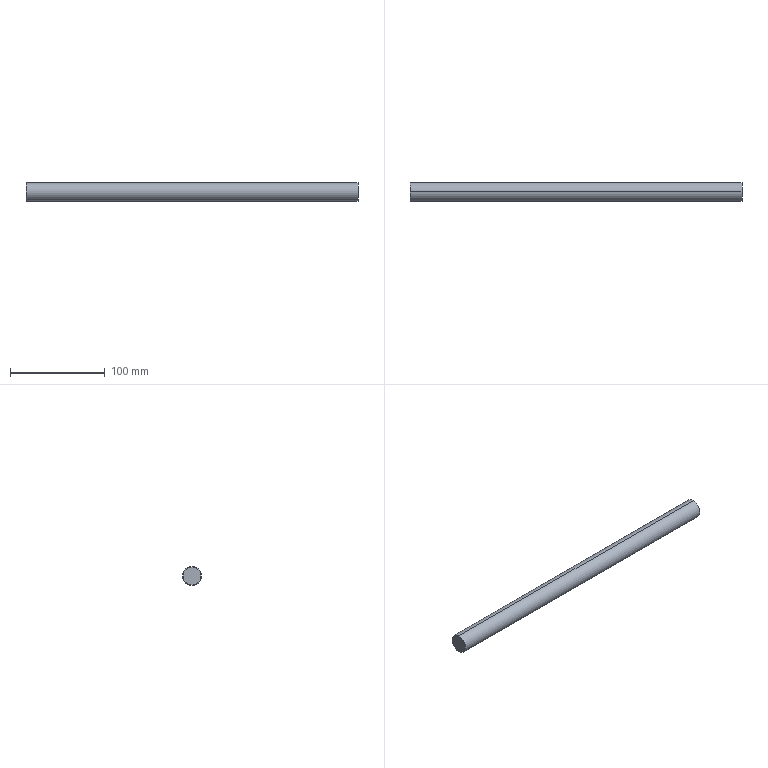Part | STEP file | Hold-down sync guide rod | 1 solid | 10 faces | box 350 x 20 x 20 mm | volume 109206 mm3 | cylinder 4 | cone 4 | plane 2 | commonest cylinder face diameters 6.8 x2 20 x2
STEP:
#1=CARTESIAN_POINT('',(0.,0.,0.));
#2=DIRECTION('',(0.,0.,1.));
#3=DIRECTION('',(1.,0.,0.));
#4=AXIS2_PLACEMENT_3D('',#1,#2,#3);
#5=CARTESIAN_POINT('',(330.25,18.056,30.521));
#6=VERTEX_POINT('',#5);
#7=CARTESIAN_POINT('',(350.,18.056,30.521));
#8=VERTEX_POINT('',#7);
#9=CARTESIAN_POINT('',(350.,18.056,30.521));
#10=DIRECTION('',(1.,0.,0.));
#11=VECTOR('',#10,1.);
#12=LINE('',#9,#11);
#13=CARTESIAN_POINT('',(350.,18.056,33.921));
#14=DIRECTION('',(1.,0.,0.));
#15=DIRECTION('',(0.,0.,-1.));
#16=AXIS2_PLACEMENT_3D('',#13,#14,#15);
#17=CYLINDRICAL_SURFACE('',#16,3.4);
#18=CARTESIAN_POINT('',(6.283,0.));
#19=DIRECTION('',(0.,1.));
#20=VECTOR('',#19,1.);
#21=LINE('',#18,#20);
#22=(GEOMETRIC_REPRESENTATION_CONTEXT(2)PARAMETRIC_REPRESENTATION_CONTEXT()REPRESENTATION_CONTEXT('',''));
#23=DEFINITIONAL_REPRESENTATION('',(#21),#22);
#24=PCURVE('',#17,#23);
#25=CARTESIAN_POINT('',(350.,18.056,33.921));
#26=DIRECTION('',(1.,0.,0.));
#27=DIRECTION('',(0.,0.,-1.));
#28=AXIS2_PLACEMENT_3D('',#25,#26,#27);
#29=CYLINDRICAL_SURFACE('',#28,3.4);
#30=CARTESIAN_POINT('',(0.,0.));
#31=DIRECTION('',(0.,1.));
#32=VECTOR('',#31,1.);
#33=LINE('',#30,#32);
#34=(GEOMETRIC_REPRESENTATION_CONTEXT(2)PARAMETRIC_REPRESENTATION_CONTEXT()REPRESENTATION_CONTEXT('',''));
#35=DEFINITIONAL_REPRESENTATION('',(#33),#34);
#36=PCURVE('',#29,#35);
#37=SURFACE_CURVE('',#12,(#24,#36),.PCURVE_S1.);
#38=EDGE_CURVE('',#6,#8,#37,.T.);
#39=ORIENTED_EDGE('',*,*,#38,.T.);
#40=CARTESIAN_POINT('',(350.,18.056,37.321));
#41=VERTEX_POINT('',#40);
#42=CARTESIAN_POINT('',(350.,18.056,33.921));
#43=DIRECTION('',(1.,0.,0.));
#44=DIRECTION('',(0.,0.,-1.));
#45=AXIS2_PLACEMENT_3D('',#42,#43,#44);
#46=CIRCLE('',#45,3.4);
#47=CARTESIAN_POINT('',(0.,0.));
#48=DIRECTION('',(1.,0.));
#49=VECTOR('',#48,1.);
#50=LINE('',#47,#49);
#51=(GEOMETRIC_REPRESENTATION_CONTEXT(2)PARAMETRIC_REPRESENTATION_CONTEXT()REPRESENTATION_CONTEXT('',''));
#52=DEFINITIONAL_REPRESENTATION('',(#50),#51);
#53=PCURVE('',#17,#52);
#54=CARTESIAN_POINT('',(350.,18.056,33.921));
#55=DIRECTION('',(1.,0.,0.));
#56=DIRECTION('',(0.,0.,-1.));
#57=AXIS2_PLACEMENT_3D('',#54,#55,#56);
#58=PLANE('',#57);
#59=CARTESIAN_POINT('',(0.,0.));
#60=DIRECTION('',(1.,0.));
#61=AXIS2_PLACEMENT_2D('',#59,#60);
#62=CIRCLE('',#61,3.4);
#63=(GEOMETRIC_REPRESENTATION_CONTEXT(2)PARAMETRIC_REPRESENTATION_CONTEXT()REPRESENTATION_CONTEXT('',''));
#64=DEFINITIONAL_REPRESENTATION('',(#62),#63);
#65=PCURVE('',#58,#64);
#66=SURFACE_CURVE('',#46,(#53,#65),.PCURVE_S1.);
#67=EDGE_CURVE('',#41,#8,#66,.T.);
#68=ORIENTED_EDGE('',*,*,#67,.F.);
#69=CARTESIAN_POINT('',(330.25,18.056,37.321));
#70=VERTEX_POINT('',#69);
#71=CARTESIAN_POINT('',(350.,18.056,37.321));
#72=DIRECTION('',(1.,0.,0.));
#73=VECTOR('',#72,1.);
#74=LINE('',#71,#73);
#75=CARTESIAN_POINT('',(3.142,0.));
#76=DIRECTION('',(0.,1.));
#77=VECTOR('',#76,1.);
#78=LINE('',#75,#77);
#79=(GEOMETRIC_REPRESENTATION_CONTEXT(2)PARAMETRIC_REPRESENTATION_CONTEXT()REPRESENTATION_CONTEXT('',''));
#80=DEFINITIONAL_REPRESENTATION('',(#78),#79);
#81=PCURVE('',#17,#80);
#82=CARTESIAN_POINT('',(3.142,0.));
#83=DIRECTION('',(0.,1.));
#84=VECTOR('',#83,1.);
#85=LINE('',#82,#84);
#86=(GEOMETRIC_REPRESENTATION_CONTEXT(2)PARAMETRIC_REPRESENTATION_CONTEXT()REPRESENTATION_CONTEXT('',''));
#87=DEFINITIONAL_REPRESENTATION('',(#85),#86);
#88=PCURVE('',#29,#87);
#89=SURFACE_CURVE('',#74,(#81,#88),.PCURVE_S1.);
#90=EDGE_CURVE('',#70,#41,#89,.T.);
#91=ORIENTED_EDGE('',*,*,#90,.F.);
#92=CARTESIAN_POINT('',(330.25,18.056,33.921));
#93=DIRECTION('',(1.,0.,0.));
#94=DIRECTION('',(0.,0.,-1.));
#95=AXIS2_PLACEMENT_3D('',#92,#93,#94);
#96=CIRCLE('',#95,3.4);
#97=CARTESIAN_POINT('',(0.,-19.75));
#98=DIRECTION('',(1.,0.));
#99=VECTOR('',#98,1.);
#100=LINE('',#97,#99);
#101=(GEOMETRIC_REPRESENTATION_CONTEXT(2)PARAMETRIC_REPRESENTATION_CONTEXT()REPRESENTATION_CONTEXT('',''));
#102=DEFINITIONAL_REPRESENTATION('',(#100),#101);
#103=PCURVE('',#17,#102);
#104=CARTESIAN_POINT('',(330.25,18.056,33.921));
#105=DIRECTION('',(1.,0.,0.));
#106=DIRECTION('',(0.,0.,-1.));
#107=AXIS2_PLACEMENT_3D('',#104,#105,#106);
#108=CONICAL_SURFACE('',#107,3.4,1.03);
#109=CARTESIAN_POINT('',(0.,0.));
#110=DIRECTION('',(1.,0.));
#111=VECTOR('',#110,1.);
#112=LINE('',#109,#111);
#113=(GEOMETRIC_REPRESENTATION_CONTEXT(2)PARAMETRIC_REPRESENTATION_CONTEXT()REPRESENTATION_CONTEXT('',''));
#114=DEFINITIONAL_REPRESENTATION('',(#112),#113);
#115=PCURVE('',#108,#114);
#116=SURFACE_CURVE('',#96,(#103,#115),.PCURVE_S1.);
#117=EDGE_CURVE('',#70,#6,#116,.T.);
#118=ORIENTED_EDGE('',*,*,#117,.T.);
#119=EDGE_LOOP('',(#39,#68,#91,#118));
#120=FACE_BOUND('',#119,.F.);
#121=ADVANCED_FACE('',(#120),#17,.F.);
#122=ORIENTED_EDGE('',*,*,#117,.F.);
#123=CARTESIAN_POINT('',(328.207,18.056,33.921));
#124=VERTEX_POINT('',#123);
#125=CARTESIAN_POINT('',(330.25,18.056,37.321));
#126=DIRECTION('',(0.515,0.,0.8572));
#127=VECTOR('',#126,1.);
#128=LINE('',#125,#127);
#129=CARTESIAN_POINT('',(3.142,0.));
#130=DIRECTION('',(0.,1.));
#131=VECTOR('',#130,1.);
#132=LINE('',#129,#131);
#133=(GEOMETRIC_REPRESENTATION_CONTEXT(2)PARAMETRIC_REPRESENTATION_CONTEXT()REPRESENTATION_CONTEXT('',''));
#134=DEFINITIONAL_REPRESENTATION('',(#132),#133);
#135=PCURVE('',#108,#134);
#136=CARTESIAN_POINT('',(330.25,18.056,33.921));
#137=DIRECTION('',(1.,0.,0.));
#138=DIRECTION('',(0.,0.,-1.));
#139=AXIS2_PLACEMENT_3D('',#136,#137,#138);
#140=CONICAL_SURFACE('',#139,3.4,1.03);
#141=CARTESIAN_POINT('',(3.142,0.));
#142=DIRECTION('',(0.,1.));
#143=VECTOR('',#142,1.);
#144=LINE('',#141,#143);
#145=(GEOMETRIC_REPRESENTATION_CONTEXT(2)PARAMETRIC_REPRESENTATION_CONTEXT()REPRESENTATION_CONTEXT('',''));
#146=DEFINITIONAL_REPRESENTATION('',(#144),#145);
#147=PCURVE('',#140,#146);
#148=SURFACE_CURVE('',#128,(#135,#147),.PCURVE_S1.);
#149=EDGE_CURVE('',#124,#70,#148,.T.);
#150=ORIENTED_EDGE('',*,*,#149,.F.);
#151=CARTESIAN_POINT('',(330.25,18.056,30.521));
#152=DIRECTION('',(0.515,0.,-0.8572));
#153=VECTOR('',#152,1.);
#154=LINE('',#151,#153);
#155=CARTESIAN_POINT('',(6.283,0.));
#156=DIRECTION('',(0.,1.));
#157=VECTOR('',#156,1.);
#158=LINE('',#155,#157);
#159=(GEOMETRIC_REPRESENTATION_CONTEXT(2)PARAMETRIC_REPRESENTATION_CONTEXT()REPRESENTATION_CONTEXT('',''));
#160=DEFINITIONAL_REPRESENTATION('',(#158),#159);
#161=PCURVE('',#108,#160);
#162=CARTESIAN_POINT('',(0.,0.));
#163=DIRECTION('',(0.,1.));
#164=VECTOR('',#163,1.);
#165=LINE('',#162,#164);
#166=(GEOMETRIC_REPRESENTATION_CONTEXT(2)PARAMETRIC_REPRESENTATION_CONTEXT()REPRESENTATION_CONTEXT('',''));
#167=DEFINITIONAL_REPRESENTATION('',(#165),#166);
#168=PCURVE('',#140,#167);
#169=SURFACE_CURVE('',#154,(#161,#168),.PCURVE_S1.);
#170=EDGE_CURVE('',#124,#6,#169,.T.);
#171=ORIENTED_EDGE('',*,*,#170,.T.);
#172=EDGE_LOOP('',(#122,#150,#171));
#173=FACE_BOUND('',#172,.F.);
#174=ADVANCED_FACE('',(#173),#108,.F.);
#175=CARTESIAN_POINT('',(0.,18.056,43.421));
#176=VERTEX_POINT('',#175);
#177=CARTESIAN_POINT('',(0.,18.056,24.421));
#178=VERTEX_POINT('',#177);
#179=CARTESIAN_POINT('',(0.,18.056,33.921));
#180=DIRECTION('',(-1.,0.,0.));
#181=DIRECTION('',(0.,0.,-1.));
#182=AXIS2_PLACEMENT_3D('',#179,#180,#181);
#183=CIRCLE('',#182,9.5);
#184=CARTESIAN_POINT('',(0.5,18.056,33.921));
#185=DIRECTION('',(1.,0.,0.));
#186=DIRECTION('',(0.,0.,-1.));
#187=AXIS2_PLACEMENT_3D('',#184,#185,#186);
#188=CONICAL_SURFACE('',#187,10.,0.7854);
#189=CARTESIAN_POINT('',(6.283,-0.5));
#190=DIRECTION('',(-1.,0.));
#191=VECTOR('',#190,1.);
#192=LINE('',#189,#191);
#193=(GEOMETRIC_REPRESENTATION_CONTEXT(2)PARAMETRIC_REPRESENTATION_CONTEXT()REPRESENTATION_CONTEXT('',''));
#194=DEFINITIONAL_REPRESENTATION('',(#192),#193);
#195=PCURVE('',#188,#194);
#196=CARTESIAN_POINT('',(0.,18.056,33.921));
#197=DIRECTION('',(1.,0.,0.));
#198=DIRECTION('',(0.,0.,-1.));
#199=AXIS2_PLACEMENT_3D('',#196,#197,#198);
#200=PLANE('',#199);
#201=CARTESIAN_POINT('',(9.5,0.));
#202=CARTESIAN_POINT('',(9.5,-16.454));
#203=CARTESIAN_POINT('',(-4.75,-8.227));
#204=CARTESIAN_POINT('',(-19.,0.));
#205=CARTESIAN_POINT('',(-4.75,8.227));
#206=CARTESIAN_POINT('',(9.5,16.454));
#207=CARTESIAN_POINT('',(9.5,0.));
#208=(BOUNDED_CURVE()B_SPLINE_CURVE(2,(#201,#202,#203,#204,#205,#206,#207),.UNSPECIFIED.,.T.,.F.)B_SPLINE_CURVE_WITH_KNOTS((1,2,2,2,2,1),(-2.094,0.,2.094,4.189,6.283,8.378),.UNSPECIFIED.)CURVE()GEOMETRIC_REPRESENTATION_ITEM()RATIONAL_B_SPLINE_CURVE((1.,0.5,1.,0.5,1.,0.5,1.))REPRESENTATION_ITEM(''));
#209=(GEOMETRIC_REPRESENTATION_CONTEXT(2)PARAMETRIC_REPRESENTATION_CONTEXT()REPRESENTATION_CONTEXT('',''));
#210=DEFINITIONAL_REPRESENTATION('',(#208),#209);
#211=PCURVE('',#200,#210);
#212=SURFACE_CURVE('',#183,(#195,#211),.PCURVE_S1.);
#213=EDGE_CURVE('',#176,#178,#212,.T.);
#214=ORIENTED_EDGE('',*,*,#213,.F.);
#215=CARTESIAN_POINT('',(0.5,18.056,43.921));
#216=VERTEX_POINT('',#215);
#217=CARTESIAN_POINT('',(0.5,18.056,43.921));
#218=DIRECTION('',(0.7071,0.,0.7071));
#219=VECTOR('',#218,1.);
#220=LINE('',#217,#219);
#221=CARTESIAN_POINT('',(3.142,0.));
#222=DIRECTION('',(0.,1.));
#223=VECTOR('',#222,1.);
#224=LINE('',#221,#223);
#225=(GEOMETRIC_REPRESENTATION_CONTEXT(2)PARAMETRIC_REPRESENTATION_CONTEXT()REPRESENTATION_CONTEXT('',''));
#226=DEFINITIONAL_REPRESENTATION('',(#224),#225);
#227=PCURVE('',#188,#226);
#228=CARTESIAN_POINT('',(0.5,18.056,33.921));
#229=DIRECTION('',(1.,0.,0.));
#230=DIRECTION('',(0.,0.,-1.));
#231=AXIS2_PLACEMENT_3D('',#228,#229,#230);
#232=CONICAL_SURFACE('',#231,10.,0.7854);
#233=CARTESIAN_POINT('',(3.142,0.));
#234=DIRECTION('',(0.,1.));
#235=VECTOR('',#234,1.);
#236=LINE('',#233,#235);
#237=(GEOMETRIC_REPRESENTATION_CONTEXT(2)PARAMETRIC_REPRESENTATION_CONTEXT()REPRESENTATION_CONTEXT('',''));
#238=DEFINITIONAL_REPRESENTATION('',(#236),#237);
#239=PCURVE('',#232,#238);
#240=SURFACE_CURVE('',#220,(#227,#239),.PCURVE_S1.);
#241=EDGE_CURVE('',#176,#216,#240,.T.);
#242=ORIENTED_EDGE('',*,*,#241,.T.);
#243=CARTESIAN_POINT('',(0.5,18.056,23.921));
#244=VERTEX_POINT('',#243);
#245=CARTESIAN_POINT('',(0.5,18.056,33.921));
#246=DIRECTION('',(1.,0.,0.));
#247=DIRECTION('',(0.,0.,-1.));
#248=AXIS2_PLACEMENT_3D('',#245,#246,#247);
#249=CIRCLE('',#248,10.);
#250=CARTESIAN_POINT('',(0.,0.));
#251=DIRECTION('',(1.,0.));
#252=VECTOR('',#251,1.);
#253=LINE('',#250,#252);
#254=(GEOMETRIC_REPRESENTATION_CONTEXT(2)PARAMETRIC_REPRESENTATION_CONTEXT()REPRESENTATION_CONTEXT('',''));
#255=DEFINITIONAL_REPRESENTATION('',(#253),#254);
#256=PCURVE('',#188,#255);
#257=CARTESIAN_POINT('',(350.,18.056,33.921));
#258=DIRECTION('',(-1.,0.,0.));
#259=DIRECTION('',(0.,0.,1.));
#260=AXIS2_PLACEMENT_3D('',#257,#258,#259);
#261=CYLINDRICAL_SURFACE('',#260,10.);
#262=CARTESIAN_POINT('',(3.142,349.5));
#263=DIRECTION('',(-1.,0.));
#264=VECTOR('',#263,1.);
#265=LINE('',#262,#264);
#266=(GEOMETRIC_REPRESENTATION_CONTEXT(2)PARAMETRIC_REPRESENTATION_CONTEXT()REPRESENTATION_CONTEXT('',''));
#267=DEFINITIONAL_REPRESENTATION('',(#265),#266);
#268=PCURVE('',#261,#267);
#269=SURFACE_CURVE('',#249,(#256,#268),.PCURVE_S1.);
#270=EDGE_CURVE('',#244,#216,#269,.T.);
#271=ORIENTED_EDGE('',*,*,#270,.F.);
#272=CARTESIAN_POINT('',(0.5,18.056,23.921));
#273=DIRECTION('',(0.7071,0.,-0.7071));
#274=VECTOR('',#273,1.);
#275=LINE('',#272,#274);
#276=CARTESIAN_POINT('',(0.,0.));
#277=DIRECTION('',(0.,1.));
#278=VECTOR('',#277,1.);
#279=LINE('',#276,#278);
#280=(GEOMETRIC_REPRESENTATION_CONTEXT(2)PARAMETRIC_REPRESENTATION_CONTEXT()REPRESENTATION_CONTEXT('',''));
#281=DEFINITIONAL_REPRESENTATION('',(#279),#280);
#282=PCURVE('',#188,#281);
#283=CARTESIAN_POINT('',(6.283,0.));
#284=DIRECTION('',(0.,1.));
#285=VECTOR('',#284,1.);
#286=LINE('',#283,#285);
#287=(GEOMETRIC_REPRESENTATION_CONTEXT(2)PARAMETRIC_REPRESENTATION_CONTEXT()REPRESENTATION_CONTEXT('',''));
#288=DEFINITIONAL_REPRESENTATION('',(#286),#287);
#289=PCURVE('',#232,#288);
#290=SURFACE_CURVE('',#275,(#282,#289),.PCURVE_S1.);
#291=EDGE_CURVE('',#178,#244,#290,.T.);
#292=ORIENTED_EDGE('',*,*,#291,.F.);
#293=EDGE_LOOP('',(#214,#242,#271,#292));
#294=FACE_BOUND('',#293,.T.);
#295=ADVANCED_FACE('',(#294),#188,.T.);
#296=CARTESIAN_POINT('',(350.,18.056,23.921));
#297=VERTEX_POINT('',#296);
#298=CARTESIAN_POINT('',(350.,18.056,43.921));
#299=VERTEX_POINT('',#298);
#300=CARTESIAN_POINT('',(350.,18.056,33.921));
#301=DIRECTION('',(1.,0.,0.));
#302=DIRECTION('',(0.,0.,-1.));
#303=AXIS2_PLACEMENT_3D('',#300,#301,#302);
#304=CIRCLE('',#303,10.);
#305=CARTESIAN_POINT('',(3.142,0.));
#306=DIRECTION('',(-1.,0.));
#307=VECTOR('',#306,1.);
#308=LINE('',#305,#307);
#309=(GEOMETRIC_REPRESENTATION_CONTEXT(2)PARAMETRIC_REPRESENTATION_CONTEXT()REPRESENTATION_CONTEXT('',''));
#310=DEFINITIONAL_REPRESENTATION('',(#308),#309);
#311=PCURVE('',#261,#310);
#312=CARTESIAN_POINT('',(0.,0.));
#313=DIRECTION('',(1.,0.));
#314=AXIS2_PLACEMENT_2D('',#312,#313);
#315=CIRCLE('',#314,10.);
#316=(GEOMETRIC_REPRESENTATION_CONTEXT(2)PARAMETRIC_REPRESENTATION_CONTEXT()REPRESENTATION_CONTEXT('',''));
#317=DEFINITIONAL_REPRESENTATION('',(#315),#316);
#318=PCURVE('',#58,#317);
#319=SURFACE_CURVE('',#304,(#311,#318),.PCURVE_S1.);
#320=EDGE_CURVE('',#297,#299,#319,.T.);
#321=ORIENTED_EDGE('',*,*,#320,.F.);
#322=CARTESIAN_POINT('',(350.,18.056,23.921));
#323=DIRECTION('',(-1.,0.,0.));
#324=VECTOR('',#323,1.);
#325=LINE('',#322,#324);
#326=CARTESIAN_POINT('',(3.142,0.));
#327=DIRECTION('',(0.,1.));
#328=VECTOR('',#327,1.);
#329=LINE('',#326,#328);
#330=(GEOMETRIC_REPRESENTATION_CONTEXT(2)PARAMETRIC_REPRESENTATION_CONTEXT()REPRESENTATION_CONTEXT('',''));
#331=DEFINITIONAL_REPRESENTATION('',(#329),#330);
#332=PCURVE('',#261,#331);
#333=CARTESIAN_POINT('',(350.,18.056,33.921));
#334=DIRECTION('',(-1.,0.,0.));
#335=DIRECTION('',(0.,0.,1.));
#336=AXIS2_PLACEMENT_3D('',#333,#334,#335);
#337=CYLINDRICAL_SURFACE('',#336,10.);
#338=CARTESIAN_POINT('',(3.142,0.));
#339=DIRECTION('',(0.,1.));
#340=VECTOR('',#339,1.);
#341=LINE('',#338,#340);
#342=(GEOMETRIC_REPRESENTATION_CONTEXT(2)PARAMETRIC_REPRESENTATION_CONTEXT()REPRESENTATION_CONTEXT('',''));
#343=DEFINITIONAL_REPRESENTATION('',(#341),#342);
#344=PCURVE('',#337,#343);
#345=SURFACE_CURVE('',#325,(#332,#344),.PCURVE_S1.);
#346=EDGE_CURVE('',#297,#244,#345,.T.);
#347=ORIENTED_EDGE('',*,*,#346,.T.);
#348=ORIENTED_EDGE('',*,*,#270,.T.);
#349=CARTESIAN_POINT('',(350.,18.056,43.921));
#350=DIRECTION('',(-1.,0.,0.));
#351=VECTOR('',#350,1.);
#352=LINE('',#349,#351);
#353=CARTESIAN_POINT('',(0.,0.));
#354=DIRECTION('',(0.,1.));
#355=VECTOR('',#354,1.);
#356=LINE('',#353,#355);
#357=(GEOMETRIC_REPRESENTATION_CONTEXT(2)PARAMETRIC_REPRESENTATION_CONTEXT()REPRESENTATION_CONTEXT('',''));
#358=DEFINITIONAL_REPRESENTATION('',(#356),#357);
#359=PCURVE('',#261,#358);
#360=CARTESIAN_POINT('',(6.283,0.));
#361=DIRECTION('',(0.,1.));
#362=VECTOR('',#361,1.);
#363=LINE('',#360,#362);
#364=(GEOMETRIC_REPRESENTATION_CONTEXT(2)PARAMETRIC_REPRESENTATION_CONTEXT()REPRESENTATION_CONTEXT('',''));
#365=DEFINITIONAL_REPRESENTATION('',(#363),#364);
#366=PCURVE('',#337,#365);
#367=SURFACE_CURVE('',#352,(#359,#366),.PCURVE_S1.);
#368=EDGE_CURVE('',#299,#216,#367,.T.);
#369=ORIENTED_EDGE('',*,*,#368,.F.);
#370=EDGE_LOOP('',(#321,#347,#348,#369));
#371=FACE_BOUND('',#370,.T.);
#372=ADVANCED_FACE('',(#371),#261,.T.);
#373=ORIENTED_EDGE('',*,*,#346,.F.);
#374=CARTESIAN_POINT('',(350.,18.056,33.921));
#375=DIRECTION('',(1.,0.,0.));
#376=DIRECTION('',(0.,0.,-1.));
#377=AXIS2_PLACEMENT_3D('',#374,#375,#376);
#378=CIRCLE('',#377,10.);
#379=CARTESIAN_POINT('',(9.425,0.));
#380=DIRECTION('',(-1.,0.));
#381=VECTOR('',#380,1.);
#382=LINE('',#379,#381);
#383=(GEOMETRIC_REPRESENTATION_CONTEXT(2)PARAMETRIC_REPRESENTATION_CONTEXT()REPRESENTATION_CONTEXT('',''));
#384=DEFINITIONAL_REPRESENTATION('',(#382),#383);
#385=PCURVE('',#337,#384);
#386=CARTESIAN_POINT('',(0.,0.));
#387=DIRECTION('',(1.,0.));
#388=AXIS2_PLACEMENT_2D('',#386,#387);
#389=CIRCLE('',#388,10.);
#390=(GEOMETRIC_REPRESENTATION_CONTEXT(2)PARAMETRIC_REPRESENTATION_CONTEXT()REPRESENTATION_CONTEXT('',''));
#391=DEFINITIONAL_REPRESENTATION('',(#389),#390);
#392=PCURVE('',#58,#391);
#393=SURFACE_CURVE('',#378,(#385,#392),.PCURVE_S1.);
#394=EDGE_CURVE('',#299,#297,#393,.T.);
#395=ORIENTED_EDGE('',*,*,#394,.F.);
#396=ORIENTED_EDGE('',*,*,#368,.T.);
#397=CARTESIAN_POINT('',(0.5,18.056,33.921));
#398=DIRECTION('',(1.,0.,0.));
#399=DIRECTION('',(0.,0.,-1.));
#400=AXIS2_PLACEMENT_3D('',#397,#398,#399);
#401=CIRCLE('',#400,10.);
#402=CARTESIAN_POINT('',(9.425,349.5));
#403=DIRECTION('',(-1.,0.));
#404=VECTOR('',#403,1.);
#405=LINE('',#402,#404);
#406=(GEOMETRIC_REPRESENTATION_CONTEXT(2)PARAMETRIC_REPRESENTATION_CONTEXT()REPRESENTATION_CONTEXT('',''));
#407=DEFINITIONAL_REPRESENTATION('',(#405),#406);
#408=PCURVE('',#337,#407);
#409=CARTESIAN_POINT('',(0.,0.));
#410=DIRECTION('',(1.,0.));
#411=VECTOR('',#410,1.);
#412=LINE('',#409,#411);
#413=(GEOMETRIC_REPRESENTATION_CONTEXT(2)PARAMETRIC_REPRESENTATION_CONTEXT()REPRESENTATION_CONTEXT('',''));
#414=DEFINITIONAL_REPRESENTATION('',(#412),#413);
#415=PCURVE('',#232,#414);
#416=SURFACE_CURVE('',#401,(#408,#415),.PCURVE_S1.);
#417=EDGE_CURVE('',#216,#244,#416,.T.);
#418=ORIENTED_EDGE('',*,*,#417,.T.);
#419=EDGE_LOOP('',(#373,#395,#396,#418));
#420=FACE_BOUND('',#419,.T.);
#421=ADVANCED_FACE('',(#420),#337,.T.);
#422=CARTESIAN_POINT('',(350.,18.056,33.921));
#423=DIRECTION('',(1.,0.,0.));
#424=DIRECTION('',(0.,0.,-1.));
#425=AXIS2_PLACEMENT_3D('',#422,#423,#424);
#426=CIRCLE('',#425,3.4);
#427=CARTESIAN_POINT('',(0.,0.));
#428=DIRECTION('',(1.,0.));
#429=AXIS2_PLACEMENT_2D('',#427,#428);
#430=CIRCLE('',#429,3.4);
#431=(GEOMETRIC_REPRESENTATION_CONTEXT(2)PARAMETRIC_REPRESENTATION_CONTEXT()REPRESENTATION_CONTEXT('',''));
#432=DEFINITIONAL_REPRESENTATION('',(#430),#431);
#433=PCURVE('',#58,#432);
#434=CARTESIAN_POINT('',(0.,0.));
#435=DIRECTION('',(1.,0.));
#436=VECTOR('',#435,1.);
#437=LINE('',#434,#436);
#438=(GEOMETRIC_REPRESENTATION_CONTEXT(2)PARAMETRIC_REPRESENTATION_CONTEXT()REPRESENTATION_CONTEXT('',''));
#439=DEFINITIONAL_REPRESENTATION('',(#437),#438);
#440=PCURVE('',#29,#439);
#441=SURFACE_CURVE('',#426,(#433,#440),.PCURVE_S1.);
#442=EDGE_CURVE('',#8,#41,#441,.T.);
#443=ORIENTED_EDGE('',*,*,#442,.F.);
#444=ORIENTED_EDGE('',*,*,#67,.F.);
#445=EDGE_LOOP('',(#443,#444));
#446=FACE_BOUND('',#445,.T.);
#447=ORIENTED_EDGE('',*,*,#394,.T.);
#448=ORIENTED_EDGE('',*,*,#320,.T.);
#449=EDGE_LOOP('',(#447,#448));
#450=FACE_BOUND('',#449,.T.);
#451=ADVANCED_FACE('',(#446,#450),#58,.T.);
#452=CARTESIAN_POINT('',(0.,18.056,33.921));
#453=DIRECTION('',(-1.,0.,0.));
#454=DIRECTION('',(0.,0.,-1.));
#455=AXIS2_PLACEMENT_3D('',#452,#453,#454);
#456=CIRCLE('',#455,9.5);
#457=CARTESIAN_POINT('',(9.5,0.));
#458=CARTESIAN_POINT('',(9.5,-16.454));
#459=CARTESIAN_POINT('',(-4.75,-8.227));
#460=CARTESIAN_POINT('',(-19.,0.));
#461=CARTESIAN_POINT('',(-4.75,8.227));
#462=CARTESIAN_POINT('',(9.5,16.454));
#463=CARTESIAN_POINT('',(9.5,0.));
#464=(BOUNDED_CURVE()B_SPLINE_CURVE(2,(#457,#458,#459,#460,#461,#462,#463),.UNSPECIFIED.,.T.,.F.)B_SPLINE_CURVE_WITH_KNOTS((1,2,2,2,2,1),(-2.094,0.,2.094,4.189,6.283,8.378),.UNSPECIFIED.)CURVE()GEOMETRIC_REPRESENTATION_ITEM()RATIONAL_B_SPLINE_CURVE((1.,0.5,1.,0.5,1.,0.5,1.))REPRESENTATION_ITEM(''));
#465=(GEOMETRIC_REPRESENTATION_CONTEXT(2)PARAMETRIC_REPRESENTATION_CONTEXT()REPRESENTATION_CONTEXT('',''));
#466=DEFINITIONAL_REPRESENTATION('',(#464),#465);
#467=PCURVE('',#200,#466);
#468=CARTESIAN_POINT('',(6.283,-0.5));
#469=DIRECTION('',(-1.,0.));
#470=VECTOR('',#469,1.);
#471=LINE('',#468,#470);
#472=(GEOMETRIC_REPRESENTATION_CONTEXT(2)PARAMETRIC_REPRESENTATION_CONTEXT()REPRESENTATION_CONTEXT('',''));
#473=DEFINITIONAL_REPRESENTATION('',(#471),#472);
#474=PCURVE('',#232,#473);
#475=SURFACE_CURVE('',#456,(#467,#474),.PCURVE_S1.);
#476=EDGE_CURVE('',#178,#176,#475,.T.);
#477=ORIENTED_EDGE('',*,*,#476,.T.);
#478=ORIENTED_EDGE('',*,*,#213,.T.);
#479=EDGE_LOOP('',(#477,#478));
#480=FACE_BOUND('',#479,.T.);
#481=ADVANCED_FACE('',(#480),#200,.F.);
#482=ORIENTED_EDGE('',*,*,#241,.F.);
#483=ORIENTED_EDGE('',*,*,#476,.F.);
#484=ORIENTED_EDGE('',*,*,#291,.T.);
#485=ORIENTED_EDGE('',*,*,#417,.F.);
#486=EDGE_LOOP('',(#482,#483,#484,#485));
#487=FACE_BOUND('',#486,.T.);
#488=ADVANCED_FACE('',(#487),#232,.T.);
#489=CARTESIAN_POINT('',(330.25,18.056,33.921));
#490=DIRECTION('',(1.,0.,0.));
#491=DIRECTION('',(0.,0.,-1.));
#492=AXIS2_PLACEMENT_3D('',#489,#490,#491);
#493=CIRCLE('',#492,3.4);
#494=CARTESIAN_POINT('',(0.,0.));
#495=DIRECTION('',(1.,0.));
#496=VECTOR('',#495,1.);
#497=LINE('',#494,#496);
#498=(GEOMETRIC_REPRESENTATION_CONTEXT(2)PARAMETRIC_REPRESENTATION_CONTEXT()REPRESENTATION_CONTEXT('',''));
#499=DEFINITIONAL_REPRESENTATION('',(#497),#498);
#500=PCURVE('',#140,#499);
#501=CARTESIAN_POINT('',(0.,-19.75));
#502=DIRECTION('',(1.,0.));
#503=VECTOR('',#502,1.);
#504=LINE('',#501,#503);
#505=(GEOMETRIC_REPRESENTATION_CONTEXT(2)PARAMETRIC_REPRESENTATION_CONTEXT()REPRESENTATION_CONTEXT('',''));
#506=DEFINITIONAL_REPRESENTATION('',(#504),#505);
#507=PCURVE('',#29,#506);
#508=SURFACE_CURVE('',#493,(#500,#507),.PCURVE_S1.);
#509=EDGE_CURVE('',#6,#70,#508,.T.);
#510=ORIENTED_EDGE('',*,*,#509,.F.);
#511=ORIENTED_EDGE('',*,*,#170,.F.);
#512=ORIENTED_EDGE('',*,*,#149,.T.);
#513=EDGE_LOOP('',(#510,#511,#512));
#514=FACE_BOUND('',#513,.F.);
#515=ADVANCED_FACE('',(#514),#140,.F.);
#516=ORIENTED_EDGE('',*,*,#442,.F.);
#517=ORIENTED_EDGE('',*,*,#38,.F.);
#518=ORIENTED_EDGE('',*,*,#509,.T.);
#519=ORIENTED_EDGE('',*,*,#90,.T.);
#520=EDGE_LOOP('',(#516,#517,#518,#519));
#521=FACE_BOUND('',#520,.F.);
#522=ADVANCED_FACE('',(#521),#29,.F.);
#523=CLOSED_SHELL('',(#121,#174,#295,#372,#421,#451,#481,#488,#515,#522));
#524=MANIFOLD_SOLID_BREP('',#523);
#525=(LENGTH_UNIT()NAMED_UNIT(*)SI_UNIT(.MILLI.,.METRE.));
#526=UNCERTAINTY_MEASURE_WITH_UNIT(LENGTH_MEASURE(0.0000001),#525,'','');
#527=(NAMED_UNIT(*)PLANE_ANGLE_UNIT()SI_UNIT($,.RADIAN.));
#528=(NAMED_UNIT(*)SI_UNIT($,.STERADIAN.)SOLID_ANGLE_UNIT());
#529=(GEOMETRIC_REPRESENTATION_CONTEXT(3)GLOBAL_UNCERTAINTY_ASSIGNED_CONTEXT((#526))GLOBAL_UNIT_ASSIGNED_CONTEXT((#525,#527,#528))REPRESENTATION_CONTEXT('',''));
#530=ADVANCED_BREP_SHAPE_REPRESENTATION('',(#4,#524),#529);